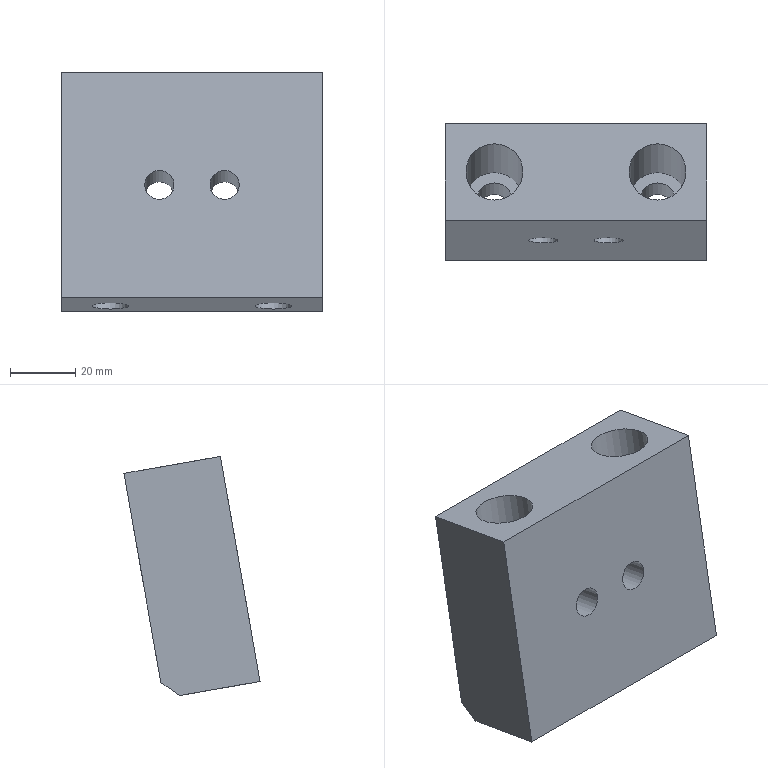Part | NX | features solid 2 | 1 solid | 19 faces | box 80 x 41.7 x 73.278 mm | volume 133522 mm3 | plane 11 | cylinder 8 | commonest cylinder face diameters 9 x2 11 x2 14 x2 17.5 x2
STEP:
#1=CARTESIAN_POINT('',(693.5,-973.128,-304.901));
#2=VERTEX_POINT('',#1);
#3=CARTESIAN_POINT('',(693.5,-997.748,-300.56));
#4=VERTEX_POINT('',#3);
#5=CARTESIAN_POINT('',(693.5,-968.204,-305.769));
#6=DIRECTION('',(0.,-0.9848,0.1736));
#7=VECTOR('',#6,1000.);
#8=LINE('',#5,#7);
#9=EDGE_CURVE('',#2,#4,#8,.T.);
#10=ORIENTED_EDGE('',*,*,#9,.T.);
#11=CARTESIAN_POINT('',(613.5,-997.748,-300.56));
#12=VERTEX_POINT('',#11);
#13=CARTESIAN_POINT('',(643.5,-997.748,-300.56));
#14=DIRECTION('',(1.,0.,0.));
#15=VECTOR('',#14,1000.);
#16=LINE('',#13,#15);
#17=EDGE_CURVE('',#12,#4,#16,.T.);
#18=ORIENTED_EDGE('',*,*,#17,.F.);
#19=CARTESIAN_POINT('',(613.5,-973.128,-304.901));
#20=VERTEX_POINT('',#19);
#21=CARTESIAN_POINT('',(613.5,-987.9,-302.296));
#22=DIRECTION('',(0.,-0.9848,0.1736));
#23=VECTOR('',#22,1000.);
#24=LINE('',#21,#23);
#25=EDGE_CURVE('',#20,#12,#24,.T.);
#26=ORIENTED_EDGE('',*,*,#25,.F.);
#27=CARTESIAN_POINT('',(643.5,-973.128,-304.901));
#28=DIRECTION('',(-1.,0.,0.));
#29=VECTOR('',#28,1000.);
#30=LINE('',#27,#29);
#31=EDGE_CURVE('',#2,#20,#30,.T.);
#32=ORIENTED_EDGE('',*,*,#31,.F.);
#33=EDGE_LOOP('',(#10,#18,#26,#32));
#34=FACE_BOUND('',#33,.T.);
#35=CARTESIAN_POINT('',(628.5,-988.392,-302.21));
#36=VERTEX_POINT('',#35);
#37=CARTESIAN_POINT('',(628.5,-982.976,-303.165));
#38=DIRECTION('',(0.,-0.1736,-0.9848));
#39=DIRECTION('',(0.,-0.9848,0.1736));
#40=AXIS2_PLACEMENT_3D('',#37,#38,#39);
#41=CIRCLE('',#40,5.5);
#42=EDGE_CURVE('',#36,#36,#41,.T.);
#43=ORIENTED_EDGE('',*,*,#42,.F.);
#44=EDGE_LOOP('',(#43));
#45=FACE_BOUND('',#44,.T.);
#46=CARTESIAN_POINT('',(678.5,-988.392,-302.21));
#47=VERTEX_POINT('',#46);
#48=CARTESIAN_POINT('',(678.5,-982.976,-303.165));
#49=DIRECTION('',(0.,-0.1736,-0.9848));
#50=DIRECTION('',(0.,-0.9848,0.1736));
#51=AXIS2_PLACEMENT_3D('',#48,#49,#50);
#52=CIRCLE('',#51,5.5);
#53=EDGE_CURVE('',#47,#47,#52,.T.);
#54=ORIENTED_EDGE('',*,*,#53,.F.);
#55=EDGE_LOOP('',(#54));
#56=FACE_BOUND('',#55,.T.);
#57=CARTESIAN_POINT('',(643.5,-987.9,-302.296));
#58=DIRECTION('',(0.,-0.1736,-0.9848));
#59=DIRECTION('',(1.,0.,0.));
#60=AXIS2_PLACEMENT_3D('',#57,#58,#59);
#61=PLANE('',#60);
#62=ADVANCED_FACE('',(#34,#45,#56),#61,.T.);
#63=CARTESIAN_POINT('',(613.5,-967.336,-300.845));
#64=VERTEX_POINT('',#63);
#65=CARTESIAN_POINT('',(613.5,-970.232,-302.873));
#66=DIRECTION('',(0.,-0.8192,-0.5736));
#67=VECTOR('',#66,1000.);
#68=LINE('',#65,#67);
#69=EDGE_CURVE('',#64,#20,#68,.T.);
#70=ORIENTED_EDGE('',*,*,#69,.T.);
#71=ORIENTED_EDGE('',*,*,#25,.T.);
#72=CARTESIAN_POINT('',(613.5,-985.593,-231.623));
#73=VERTEX_POINT('',#72);
#74=CARTESIAN_POINT('',(613.5,-988.197,-246.396));
#75=DIRECTION('',(0.,-0.1736,-0.9848));
#76=VECTOR('',#75,1000.);
#77=LINE('',#74,#76);
#78=EDGE_CURVE('',#73,#12,#77,.T.);
#79=ORIENTED_EDGE('',*,*,#78,.F.);
#80=CARTESIAN_POINT('',(613.5,-956.048,-236.833));
#81=VERTEX_POINT('',#80);
#82=CARTESIAN_POINT('',(613.5,-1116.572,-208.528));
#83=DIRECTION('',(0.,0.9848,-0.1736));
#84=VECTOR('',#83,1000.);
#85=LINE('',#82,#84);
#86=EDGE_CURVE('',#81,#73,#85,.F.);
#87=ORIENTED_EDGE('',*,*,#86,.F.);
#88=CARTESIAN_POINT('',(613.5,-966.467,-295.921));
#89=DIRECTION('',(0.,-0.1736,-0.9848));
#90=VECTOR('',#89,1000.);
#91=LINE('',#88,#90);
#92=EDGE_CURVE('',#64,#81,#91,.F.);
#93=ORIENTED_EDGE('',*,*,#92,.F.);
#94=EDGE_LOOP('',(#70,#71,#79,#87,#93));
#95=FACE_BOUND('',#94,.T.);
#96=CARTESIAN_POINT('',(613.5,-978.349,-248.132));
#97=DIRECTION('',(-1.,0.,0.));
#98=DIRECTION('',(0.,-0.1736,-0.9848));
#99=AXIS2_PLACEMENT_3D('',#96,#97,#98);
#100=PLANE('',#99);
#101=ADVANCED_FACE('',(#95),#100,.T.);
#102=CARTESIAN_POINT('',(663.5,-992.452,-270.523));
#103=VERTEX_POINT('',#102);
#104=CARTESIAN_POINT('',(663.5,-991.67,-266.092));
#105=DIRECTION('',(0.,0.9848,-0.1736));
#106=DIRECTION('',(0.,-0.1736,-0.9848));
#107=AXIS2_PLACEMENT_3D('',#104,#105,#106);
#108=CIRCLE('',#107,4.5);
#109=EDGE_CURVE('',#103,#103,#108,.T.);
#110=ORIENTED_EDGE('',*,*,#109,.T.);
#111=EDGE_LOOP('',(#110));
#112=FACE_BOUND('',#111,.T.);
#113=CARTESIAN_POINT('',(643.5,-992.452,-270.523));
#114=VERTEX_POINT('',#113);
#115=CARTESIAN_POINT('',(643.5,-991.67,-266.092));
#116=DIRECTION('',(0.,0.9848,-0.1736));
#117=DIRECTION('',(0.,-0.1736,-0.9848));
#118=AXIS2_PLACEMENT_3D('',#115,#116,#117);
#119=CIRCLE('',#118,4.5);
#120=EDGE_CURVE('',#114,#114,#119,.T.);
#121=ORIENTED_EDGE('',*,*,#120,.T.);
#122=EDGE_LOOP('',(#121));
#123=FACE_BOUND('',#122,.T.);
#124=CARTESIAN_POINT('',(693.5,-985.593,-231.623));
#125=VERTEX_POINT('',#124);
#126=CARTESIAN_POINT('',(607.5,-985.593,-231.623));
#127=DIRECTION('',(1.,0.,0.));
#128=VECTOR('',#127,1000.);
#129=LINE('',#126,#128);
#130=EDGE_CURVE('',#125,#73,#129,.F.);
#131=ORIENTED_EDGE('',*,*,#130,.T.);
#132=ORIENTED_EDGE('',*,*,#78,.T.);
#133=ORIENTED_EDGE('',*,*,#17,.T.);
#134=CARTESIAN_POINT('',(693.5,-996.012,-290.712));
#135=DIRECTION('',(0.,0.1736,0.9848));
#136=VECTOR('',#135,1000.);
#137=LINE('',#134,#136);
#138=EDGE_CURVE('',#4,#125,#137,.T.);
#139=ORIENTED_EDGE('',*,*,#138,.T.);
#140=EDGE_LOOP('',(#131,#132,#133,#139));
#141=FACE_BOUND('',#140,.T.);
#142=CARTESIAN_POINT('',(653.5,-996.012,-290.712));
#143=DIRECTION('',(0.,0.9848,-0.1736));
#144=DIRECTION('',(0.,0.1736,0.9848));
#145=AXIS2_PLACEMENT_3D('',#142,#143,#144);
#146=PLANE('',#145);
#147=ADVANCED_FACE('',(#112,#123,#141),#146,.F.);
#148=CARTESIAN_POINT('',(663.5,-960.911,-264.407));
#149=VERTEX_POINT('',#148);
#150=CARTESIAN_POINT('',(663.5,-962.126,-271.301));
#151=DIRECTION('',(0.,-0.9848,0.1736));
#152=DIRECTION('',(0.,0.1736,0.9848));
#153=AXIS2_PLACEMENT_3D('',#150,#151,#152);
#154=CIRCLE('',#153,7.);
#155=EDGE_CURVE('',#149,#149,#154,.T.);
#156=ORIENTED_EDGE('',*,*,#155,.T.);
#157=EDGE_LOOP('',(#156));
#158=FACE_BOUND('',#157,.T.);
#159=CARTESIAN_POINT('',(693.5,-967.336,-300.845));
#160=VERTEX_POINT('',#159);
#161=CARTESIAN_POINT('',(693.5,-956.048,-236.833));
#162=VERTEX_POINT('',#161);
#163=CARTESIAN_POINT('',(693.5,-966.467,-295.921));
#164=DIRECTION('',(0.,-0.1736,-0.9848));
#165=VECTOR('',#164,1000.);
#166=LINE('',#163,#165);
#167=EDGE_CURVE('',#160,#162,#166,.F.);
#168=ORIENTED_EDGE('',*,*,#167,.F.);
#169=CARTESIAN_POINT('',(653.5,-967.336,-300.845));
#170=DIRECTION('',(1.,0.,0.));
#171=VECTOR('',#170,1000.);
#172=LINE('',#169,#171);
#173=EDGE_CURVE('',#160,#64,#172,.F.);
#174=ORIENTED_EDGE('',*,*,#173,.T.);
#175=ORIENTED_EDGE('',*,*,#92,.T.);
#176=CARTESIAN_POINT('',(653.5,-956.048,-236.833));
#177=DIRECTION('',(-1.,0.,0.));
#178=VECTOR('',#177,1000.);
#179=LINE('',#176,#178);
#180=EDGE_CURVE('',#162,#81,#179,.T.);
#181=ORIENTED_EDGE('',*,*,#180,.F.);
#182=EDGE_LOOP('',(#168,#174,#175,#181));
#183=FACE_BOUND('',#182,.T.);
#184=CARTESIAN_POINT('',(643.5,-960.911,-264.407));
#185=VERTEX_POINT('',#184);
#186=CARTESIAN_POINT('',(643.5,-962.126,-271.301));
#187=DIRECTION('',(0.,-0.9848,0.1736));
#188=DIRECTION('',(0.,0.1736,0.9848));
#189=AXIS2_PLACEMENT_3D('',#186,#187,#188);
#190=CIRCLE('',#189,7.);
#191=EDGE_CURVE('',#185,#185,#190,.T.);
#192=ORIENTED_EDGE('',*,*,#191,.T.);
#193=EDGE_LOOP('',(#192));
#194=FACE_BOUND('',#193,.T.);
#195=CARTESIAN_POINT('',(653.5,-966.467,-295.921));
#196=DIRECTION('',(0.,0.9848,-0.1736));
#197=DIRECTION('',(0.,0.1736,0.9848));
#198=AXIS2_PLACEMENT_3D('',#195,#196,#197);
#199=PLANE('',#198);
#200=ADVANCED_FACE('',(#158,#183,#194),#199,.T.);
#201=CARTESIAN_POINT('',(678.5,-979.438,-232.709));
#202=VERTEX_POINT('',#201);
#203=CARTESIAN_POINT('',(678.5,-970.821,-234.228));
#204=DIRECTION('',(0.,-0.1736,-0.9848));
#205=DIRECTION('',(0.,-0.9848,0.1736));
#206=AXIS2_PLACEMENT_3D('',#203,#204,#205);
#207=CIRCLE('',#206,8.75);
#208=EDGE_CURVE('',#202,#202,#207,.F.);
#209=ORIENTED_EDGE('',*,*,#208,.F.);
#210=EDGE_LOOP('',(#209));
#211=FACE_BOUND('',#210,.T.);
#212=CARTESIAN_POINT('',(628.5,-979.438,-232.709));
#213=VERTEX_POINT('',#212);
#214=CARTESIAN_POINT('',(628.5,-970.821,-234.228));
#215=DIRECTION('',(0.,-0.1736,-0.9848));
#216=DIRECTION('',(0.,-0.9848,0.1736));
#217=AXIS2_PLACEMENT_3D('',#214,#215,#216);
#218=CIRCLE('',#217,8.75);
#219=EDGE_CURVE('',#213,#213,#218,.F.);
#220=ORIENTED_EDGE('',*,*,#219,.F.);
#221=EDGE_LOOP('',(#220));
#222=FACE_BOUND('',#221,.T.);
#223=CARTESIAN_POINT('',(693.5,-1116.572,-208.528));
#224=DIRECTION('',(0.,0.9848,-0.1736));
#225=VECTOR('',#224,1000.);
#226=LINE('',#223,#225);
#227=EDGE_CURVE('',#162,#125,#226,.F.);
#228=ORIENTED_EDGE('',*,*,#227,.F.);
#229=ORIENTED_EDGE('',*,*,#180,.T.);
#230=ORIENTED_EDGE('',*,*,#86,.T.);
#231=ORIENTED_EDGE('',*,*,#130,.F.);
#232=EDGE_LOOP('',(#228,#229,#230,#231));
#233=FACE_BOUND('',#232,.T.);
#234=CARTESIAN_POINT('',(607.5,-1116.572,-208.528));
#235=DIRECTION('',(0.,0.1736,0.9848));
#236=DIRECTION('',(-1.,0.,0.));
#237=AXIS2_PLACEMENT_3D('',#234,#235,#236);
#238=PLANE('',#237);
#239=ADVANCED_FACE('',(#211,#222,#233),#238,.T.);
#240=ORIENTED_EDGE('',*,*,#9,.F.);
#241=CARTESIAN_POINT('',(693.5,-967.336,-300.845));
#242=DIRECTION('',(0.,0.8192,0.5736));
#243=VECTOR('',#242,1000.);
#244=LINE('',#241,#243);
#245=EDGE_CURVE('',#2,#160,#244,.T.);
#246=ORIENTED_EDGE('',*,*,#245,.T.);
#247=ORIENTED_EDGE('',*,*,#167,.T.);
#248=ORIENTED_EDGE('',*,*,#227,.T.);
#249=ORIENTED_EDGE('',*,*,#138,.F.);
#250=EDGE_LOOP('',(#240,#246,#247,#248,#249));
#251=FACE_BOUND('',#250,.T.);
#252=CARTESIAN_POINT('',(693.5,-966.467,-295.921));
#253=DIRECTION('',(-1.,0.,0.));
#254=DIRECTION('',(0.,0.5,-0.866));
#255=AXIS2_PLACEMENT_3D('',#252,#253,#254);
#256=PLANE('',#255);
#257=ADVANCED_FACE('',(#251),#256,.F.);
#258=CARTESIAN_POINT('',(628.5,-974.087,-284.424));
#259=VERTEX_POINT('',#258);
#260=CARTESIAN_POINT('',(628.5,-979.503,-283.469));
#261=DIRECTION('',(0.,0.1736,0.9848));
#262=DIRECTION('',(0.,0.9848,-0.1736));
#263=AXIS2_PLACEMENT_3D('',#260,#261,#262);
#264=CIRCLE('',#263,5.5);
#265=EDGE_CURVE('',#259,#259,#264,.T.);
#266=ORIENTED_EDGE('',*,*,#265,.T.);
#267=EDGE_LOOP('',(#266));
#268=FACE_BOUND('',#267,.T.);
#269=ORIENTED_EDGE('',*,*,#42,.T.);
#270=EDGE_LOOP('',(#269));
#271=FACE_BOUND('',#270,.T.);
#272=CARTESIAN_POINT('',(628.5,-986.449,-322.861));
#273=DIRECTION('',(0.,-0.1736,-0.9848));
#274=DIRECTION('',(0.,0.9848,-0.1736));
#275=AXIS2_PLACEMENT_3D('',#272,#273,#274);
#276=CYLINDRICAL_SURFACE('',#275,5.5);
#277=ADVANCED_FACE('',(#268,#271),#276,.F.);
#278=ORIENTED_EDGE('',*,*,#265,.F.);
#279=EDGE_LOOP('',(#278));
#280=FACE_BOUND('',#279,.T.);
#281=CARTESIAN_POINT('',(628.5,-970.886,-284.988));
#282=VERTEX_POINT('',#281);
#283=CARTESIAN_POINT('',(628.5,-979.503,-283.469));
#284=DIRECTION('',(0.,0.1736,0.9848));
#285=DIRECTION('',(0.,0.9848,-0.1736));
#286=AXIS2_PLACEMENT_3D('',#283,#284,#285);
#287=CIRCLE('',#286,8.75);
#288=EDGE_CURVE('',#282,#282,#287,.T.);
#289=ORIENTED_EDGE('',*,*,#288,.T.);
#290=EDGE_LOOP('',(#289));
#291=FACE_BOUND('',#290,.T.);
#292=CARTESIAN_POINT('',(628.5,-979.503,-283.469));
#293=DIRECTION('',(0.,-0.1736,-0.9848));
#294=DIRECTION('',(0.,0.9848,-0.1736));
#295=AXIS2_PLACEMENT_3D('',#292,#293,#294);
#296=PLANE('',#295);
#297=ADVANCED_FACE('',(#280,#291),#296,.F.);
#298=ORIENTED_EDGE('',*,*,#288,.F.);
#299=EDGE_LOOP('',(#298));
#300=FACE_BOUND('',#299,.T.);
#301=ORIENTED_EDGE('',*,*,#219,.T.);
#302=EDGE_LOOP('',(#301));
#303=FACE_BOUND('',#302,.T.);
#304=CARTESIAN_POINT('',(628.5,-972.557,-244.076));
#305=DIRECTION('',(0.,-0.1736,-0.9848));
#306=DIRECTION('',(0.,0.9848,-0.1736));
#307=AXIS2_PLACEMENT_3D('',#304,#305,#306);
#308=CYLINDRICAL_SURFACE('',#307,8.75);
#309=ADVANCED_FACE('',(#300,#303),#308,.F.);
#310=CARTESIAN_POINT('',(643.5,-972.756,-273.996));
#311=VERTEX_POINT('',#310);
#312=CARTESIAN_POINT('',(643.5,-971.974,-269.565));
#313=DIRECTION('',(0.,0.9848,-0.1736));
#314=DIRECTION('',(0.,-0.1736,-0.9848));
#315=AXIS2_PLACEMENT_3D('',#312,#313,#314);
#316=CIRCLE('',#315,4.5);
#317=EDGE_CURVE('',#311,#311,#316,.T.);
#318=ORIENTED_EDGE('',*,*,#317,.T.);
#319=EDGE_LOOP('',(#318));
#320=FACE_BOUND('',#319,.T.);
#321=ORIENTED_EDGE('',*,*,#120,.F.);
#322=EDGE_LOOP('',(#321));
#323=FACE_BOUND('',#322,.T.);
#324=CARTESIAN_POINT('',(643.5,-991.67,-266.092));
#325=DIRECTION('',(0.,0.9848,-0.1736));
#326=DIRECTION('',(0.,0.1736,0.9848));
#327=AXIS2_PLACEMENT_3D('',#324,#325,#326);
#328=CYLINDRICAL_SURFACE('',#327,4.5);
#329=ADVANCED_FACE('',(#320,#323),#328,.F.);
#330=CARTESIAN_POINT('',(663.5,-972.756,-273.996));
#331=VERTEX_POINT('',#330);
#332=CARTESIAN_POINT('',(663.5,-971.974,-269.565));
#333=DIRECTION('',(0.,0.9848,-0.1736));
#334=DIRECTION('',(0.,-0.1736,-0.9848));
#335=AXIS2_PLACEMENT_3D('',#332,#333,#334);
#336=CIRCLE('',#335,4.5);
#337=EDGE_CURVE('',#331,#331,#336,.T.);
#338=ORIENTED_EDGE('',*,*,#337,.T.);
#339=EDGE_LOOP('',(#338));
#340=FACE_BOUND('',#339,.T.);
#341=ORIENTED_EDGE('',*,*,#109,.F.);
#342=EDGE_LOOP('',(#341));
#343=FACE_BOUND('',#342,.T.);
#344=CARTESIAN_POINT('',(663.5,-991.67,-266.092));
#345=DIRECTION('',(0.,0.9848,-0.1736));
#346=DIRECTION('',(0.,0.1736,0.9848));
#347=AXIS2_PLACEMENT_3D('',#344,#345,#346);
#348=CYLINDRICAL_SURFACE('',#347,4.5);
#349=ADVANCED_FACE('',(#340,#343),#348,.F.);
#350=CARTESIAN_POINT('',(678.5,-974.087,-284.424));
#351=VERTEX_POINT('',#350);
#352=CARTESIAN_POINT('',(678.5,-979.503,-283.469));
#353=DIRECTION('',(0.,0.1736,0.9848));
#354=DIRECTION('',(0.,0.9848,-0.1736));
#355=AXIS2_PLACEMENT_3D('',#352,#353,#354);
#356=CIRCLE('',#355,5.5);
#357=EDGE_CURVE('',#351,#351,#356,.T.);
#358=ORIENTED_EDGE('',*,*,#357,.T.);
#359=EDGE_LOOP('',(#358));
#360=FACE_BOUND('',#359,.T.);
#361=ORIENTED_EDGE('',*,*,#53,.T.);
#362=EDGE_LOOP('',(#361));
#363=FACE_BOUND('',#362,.T.);
#364=CARTESIAN_POINT('',(678.5,-986.449,-322.861));
#365=DIRECTION('',(0.,-0.1736,-0.9848));
#366=DIRECTION('',(0.,0.9848,-0.1736));
#367=AXIS2_PLACEMENT_3D('',#364,#365,#366);
#368=CYLINDRICAL_SURFACE('',#367,5.5);
#369=ADVANCED_FACE('',(#360,#363),#368,.F.);
#370=ORIENTED_EDGE('',*,*,#357,.F.);
#371=EDGE_LOOP('',(#370));
#372=FACE_BOUND('',#371,.T.);
#373=CARTESIAN_POINT('',(678.5,-970.886,-284.988));
#374=VERTEX_POINT('',#373);
#375=CARTESIAN_POINT('',(678.5,-979.503,-283.469));
#376=DIRECTION('',(0.,0.1736,0.9848));
#377=DIRECTION('',(0.,0.9848,-0.1736));
#378=AXIS2_PLACEMENT_3D('',#375,#376,#377);
#379=CIRCLE('',#378,8.75);
#380=EDGE_CURVE('',#374,#374,#379,.T.);
#381=ORIENTED_EDGE('',*,*,#380,.T.);
#382=EDGE_LOOP('',(#381));
#383=FACE_BOUND('',#382,.T.);
#384=CARTESIAN_POINT('',(678.5,-979.503,-283.469));
#385=DIRECTION('',(0.,-0.1736,-0.9848));
#386=DIRECTION('',(0.,0.9848,-0.1736));
#387=AXIS2_PLACEMENT_3D('',#384,#385,#386);
#388=PLANE('',#387);
#389=ADVANCED_FACE('',(#372,#383),#388,.F.);
#390=ORIENTED_EDGE('',*,*,#380,.F.);
#391=EDGE_LOOP('',(#390));
#392=FACE_BOUND('',#391,.T.);
#393=ORIENTED_EDGE('',*,*,#208,.T.);
#394=EDGE_LOOP('',(#393));
#395=FACE_BOUND('',#394,.T.);
#396=CARTESIAN_POINT('',(678.5,-972.557,-244.076));
#397=DIRECTION('',(0.,-0.1736,-0.9848));
#398=DIRECTION('',(0.,0.9848,-0.1736));
#399=AXIS2_PLACEMENT_3D('',#396,#397,#398);
#400=CYLINDRICAL_SURFACE('',#399,8.75);
#401=ADVANCED_FACE('',(#392,#395),#400,.F.);
#402=CARTESIAN_POINT('',(663.5,-973.19,-276.458));
#403=VERTEX_POINT('',#402);
#404=CARTESIAN_POINT('',(663.5,-971.974,-269.565));
#405=DIRECTION('',(0.,0.9848,-0.1736));
#406=DIRECTION('',(0.,-0.1736,-0.9848));
#407=AXIS2_PLACEMENT_3D('',#404,#405,#406);
#408=CIRCLE('',#407,7.);
#409=EDGE_CURVE('',#403,#403,#408,.T.);
#410=ORIENTED_EDGE('',*,*,#409,.F.);
#411=EDGE_LOOP('',(#410));
#412=FACE_BOUND('',#411,.T.);
#413=ORIENTED_EDGE('',*,*,#155,.F.);
#414=EDGE_LOOP('',(#413));
#415=FACE_BOUND('',#414,.T.);
#416=CARTESIAN_POINT('',(663.5,-976.898,-268.696));
#417=DIRECTION('',(0.,0.9848,-0.1736));
#418=DIRECTION('',(0.,0.1736,0.9848));
#419=AXIS2_PLACEMENT_3D('',#416,#417,#418);
#420=CYLINDRICAL_SURFACE('',#419,7.);
#421=ADVANCED_FACE('',(#412,#415),#420,.F.);
#422=ORIENTED_EDGE('',*,*,#337,.F.);
#423=EDGE_LOOP('',(#422));
#424=FACE_BOUND('',#423,.T.);
#425=ORIENTED_EDGE('',*,*,#409,.T.);
#426=EDGE_LOOP('',(#425));
#427=FACE_BOUND('',#426,.T.);
#428=CARTESIAN_POINT('',(663.5,-971.974,-269.565));
#429=DIRECTION('',(0.,-0.9848,0.1736));
#430=DIRECTION('',(0.,-0.1736,-0.9848));
#431=AXIS2_PLACEMENT_3D('',#428,#429,#430);
#432=PLANE('',#431);
#433=ADVANCED_FACE('',(#424,#427),#432,.F.);
#434=CARTESIAN_POINT('',(643.5,-973.19,-276.458));
#435=VERTEX_POINT('',#434);
#436=CARTESIAN_POINT('',(643.5,-971.974,-269.565));
#437=DIRECTION('',(0.,0.9848,-0.1736));
#438=DIRECTION('',(0.,-0.1736,-0.9848));
#439=AXIS2_PLACEMENT_3D('',#436,#437,#438);
#440=CIRCLE('',#439,7.);
#441=EDGE_CURVE('',#435,#435,#440,.T.);
#442=ORIENTED_EDGE('',*,*,#441,.F.);
#443=EDGE_LOOP('',(#442));
#444=FACE_BOUND('',#443,.T.);
#445=ORIENTED_EDGE('',*,*,#191,.F.);
#446=EDGE_LOOP('',(#445));
#447=FACE_BOUND('',#446,.T.);
#448=CARTESIAN_POINT('',(643.5,-976.898,-268.696));
#449=DIRECTION('',(0.,0.9848,-0.1736));
#450=DIRECTION('',(0.,0.1736,0.9848));
#451=AXIS2_PLACEMENT_3D('',#448,#449,#450);
#452=CYLINDRICAL_SURFACE('',#451,7.);
#453=ADVANCED_FACE('',(#444,#447),#452,.F.);
#454=ORIENTED_EDGE('',*,*,#317,.F.);
#455=EDGE_LOOP('',(#454));
#456=FACE_BOUND('',#455,.T.);
#457=ORIENTED_EDGE('',*,*,#441,.T.);
#458=EDGE_LOOP('',(#457));
#459=FACE_BOUND('',#458,.T.);
#460=CARTESIAN_POINT('',(643.5,-971.974,-269.565));
#461=DIRECTION('',(0.,-0.9848,0.1736));
#462=DIRECTION('',(0.,-0.1736,-0.9848));
#463=AXIS2_PLACEMENT_3D('',#460,#461,#462);
#464=PLANE('',#463);
#465=ADVANCED_FACE('',(#456,#459),#464,.F.);
#466=ORIENTED_EDGE('',*,*,#245,.F.);
#467=ORIENTED_EDGE('',*,*,#31,.T.);
#468=ORIENTED_EDGE('',*,*,#69,.F.);
#469=ORIENTED_EDGE('',*,*,#173,.F.);
#470=EDGE_LOOP('',(#466,#467,#468,#469));
#471=FACE_BOUND('',#470,.T.);
#472=CARTESIAN_POINT('',(653.5,-967.336,-300.845));
#473=DIRECTION('',(0.,0.5736,-0.8192));
#474=DIRECTION('',(0.,-0.8192,-0.5736));
#475=AXIS2_PLACEMENT_3D('',#472,#473,#474);
#476=PLANE('',#475);
#477=ADVANCED_FACE('',(#471),#476,.T.);
#478=CLOSED_SHELL('',(#62,#101,#147,#200,#239,#257,#277,#297,#309,#329,#349,#369,#389,#401,#421,#433,#453,#465,#477));
#479=MANIFOLD_SOLID_BREP('',#478);
#480=(LENGTH_UNIT()NAMED_UNIT(*)SI_UNIT(.MILLI.,.METRE.));
#481=UNCERTAINTY_MEASURE_WITH_UNIT(LENGTH_MEASURE(0.00001),#480,'','');
#482=(NAMED_UNIT(*)PLANE_ANGLE_UNIT()SI_UNIT($,.RADIAN.));
#483=(NAMED_UNIT(*)SI_UNIT($,.STERADIAN.)SOLID_ANGLE_UNIT());
#484=(GEOMETRIC_REPRESENTATION_CONTEXT(3)GLOBAL_UNCERTAINTY_ASSIGNED_CONTEXT((#481))GLOBAL_UNIT_ASSIGNED_CONTEXT((#480,#482,#483))REPRESENTATION_CONTEXT('',''));
#485=ADVANCED_BREP_SHAPE_REPRESENTATION('',(#479),#484);